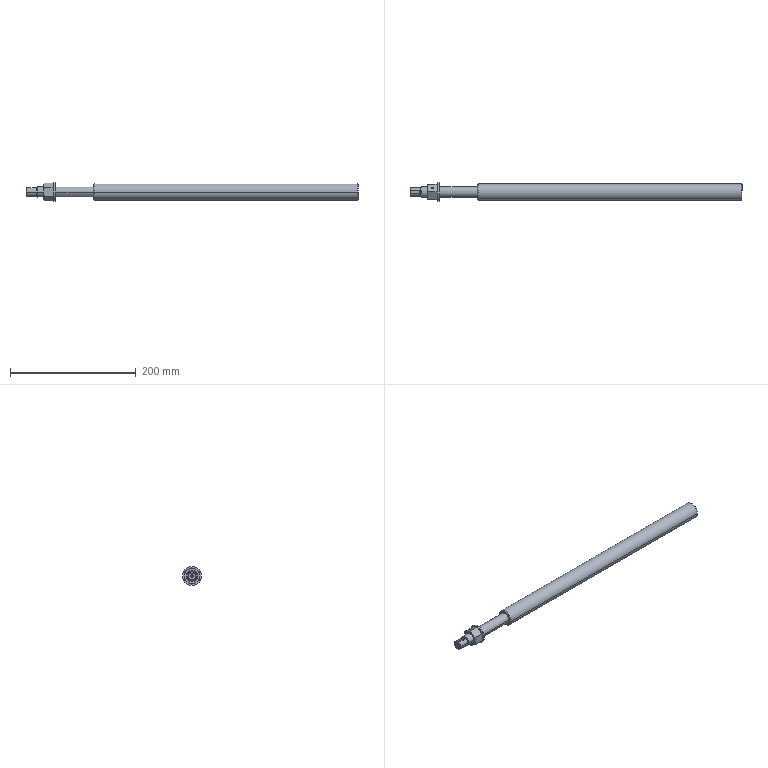Part | SolidWorks | features BaseBody 3 | 3 solids | 72 faces | box 527.001 x 30 x 30 mm | volume 250409 mm3 | cone 31 | cylinder 22 | plane 19 | commonest cylinder face diameters 4.2 x4 14 x4 16 x4 5 x2 16.5 x2 17 x2